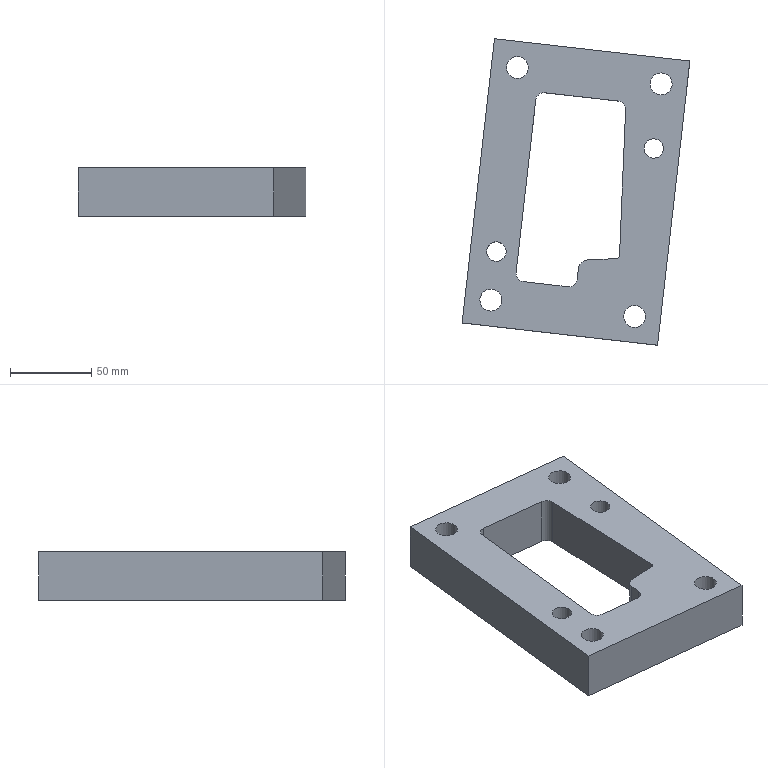Part | NX | features solid 2 | 1 solid | 36 faces | box 140.146 x 188.566 x 30 mm | volume 409846 mm3 | cylinder 18 | plane 17 | spline 1 | commonest cylinder face diameters 10 x4 13.5 x4 20 x4 12.001 x2 14.11 x2 4 x1
STEP:
#1=CARTESIAN_POINT('',(2935.529,-339.708,61.));
#2=VERTEX_POINT('',#1);
#3=CARTESIAN_POINT('',(2928.474,-339.708,61.));
#4=DIRECTION('',(0.,0.,1.));
#5=DIRECTION('',(1.,0.,0.));
#6=AXIS2_PLACEMENT_3D('',#3,#4,#5);
#7=CIRCLE('',#6,7.055);
#8=EDGE_CURVE('',#2,#2,#7,.T.);
#9=ORIENTED_EDGE('',*,*,#8,.T.);
#10=EDGE_LOOP('',(#9));
#11=FACE_BOUND('',#10,.T.);
#12=CARTESIAN_POINT('',(3032.334,-276.258,61.));
#13=VERTEX_POINT('',#12);
#14=CARTESIAN_POINT('',(3025.279,-276.258,61.));
#15=DIRECTION('',(0.,0.,1.));
#16=DIRECTION('',(1.,0.,0.));
#17=AXIS2_PLACEMENT_3D('',#14,#15,#16);
#18=CIRCLE('',#17,7.055);
#19=EDGE_CURVE('',#13,#13,#18,.T.);
#20=ORIENTED_EDGE('',*,*,#19,.T.);
#21=EDGE_LOOP('',(#20));
#22=FACE_BOUND('',#21,.T.);
#23=CARTESIAN_POINT('',(2951.315,-227.572,61.));
#24=VERTEX_POINT('',#23);
#25=CARTESIAN_POINT('',(2941.379,-226.44,61.));
#26=DIRECTION('',(0.,0.,1.));
#27=DIRECTION('',(0.9936,-0.1132,0.));
#28=AXIS2_PLACEMENT_3D('',#25,#26,#27);
#29=CIRCLE('',#28,10.);
#30=EDGE_CURVE('',#24,#24,#29,.T.);
#31=ORIENTED_EDGE('',*,*,#30,.T.);
#32=EDGE_LOOP('',(#31));
#33=FACE_BOUND('',#32,.T.);
#34=CARTESIAN_POINT('',(3039.743,-237.647,61.));
#35=VERTEX_POINT('',#34);
#36=CARTESIAN_POINT('',(3029.807,-236.515,61.));
#37=DIRECTION('',(0.,0.,1.));
#38=DIRECTION('',(0.9936,-0.1132,0.));
#39=AXIS2_PLACEMENT_3D('',#36,#37,#38);
#40=CIRCLE('',#39,10.);
#41=EDGE_CURVE('',#35,#35,#40,.T.);
#42=ORIENTED_EDGE('',*,*,#41,.T.);
#43=EDGE_LOOP('',(#42));
#44=FACE_BOUND('',#43,.T.);
#45=CARTESIAN_POINT('',(3027.592,-397.298,61.));
#46=VERTEX_POINT('',#45);
#47=CARTESIAN_POINT('',(3047.516,-222.43,61.));
#48=VERTEX_POINT('',#47);
#49=CARTESIAN_POINT('',(3037.554,-309.864,61.));
#50=DIRECTION('',(0.1132,0.9936,0.));
#51=VECTOR('',#50,1000.);
#52=LINE('',#49,#51);
#53=EDGE_CURVE('',#46,#48,#52,.T.);
#54=ORIENTED_EDGE('',*,*,#53,.F.);
#55=CARTESIAN_POINT('',(2907.37,-383.601,61.));
#56=VERTEX_POINT('',#55);
#57=CARTESIAN_POINT('',(2967.481,-390.449,61.));
#58=DIRECTION('',(0.9936,-0.1132,0.));
#59=VECTOR('',#58,1000.);
#60=LINE('',#57,#59);
#61=EDGE_CURVE('',#56,#46,#60,.T.);
#62=ORIENTED_EDGE('',*,*,#61,.F.);
#63=CARTESIAN_POINT('',(2927.293,-208.732,61.));
#64=VERTEX_POINT('',#63);
#65=CARTESIAN_POINT('',(2917.331,-296.166,61.));
#66=DIRECTION('',(-0.1132,-0.9936,0.));
#67=VECTOR('',#66,1000.);
#68=LINE('',#65,#67);
#69=EDGE_CURVE('',#64,#56,#68,.T.);
#70=ORIENTED_EDGE('',*,*,#69,.F.);
#71=CARTESIAN_POINT('',(2987.404,-215.581,61.));
#72=DIRECTION('',(-0.9936,0.1132,0.));
#73=VECTOR('',#72,1000.);
#74=LINE('',#71,#73);
#75=EDGE_CURVE('',#48,#64,#74,.T.);
#76=ORIENTED_EDGE('',*,*,#75,.F.);
#77=EDGE_LOOP('',(#54,#62,#70,#76));
#78=FACE_BOUND('',#77,.T.);
#79=CARTESIAN_POINT('',(2935.014,-370.647,61.));
#80=VERTEX_POINT('',#79);
#81=CARTESIAN_POINT('',(2925.078,-369.515,61.));
#82=DIRECTION('',(0.,0.,1.));
#83=DIRECTION('',(0.9936,-0.1132,0.));
#84=AXIS2_PLACEMENT_3D('',#81,#82,#83);
#85=CIRCLE('',#84,10.);
#86=EDGE_CURVE('',#80,#80,#85,.T.);
#87=ORIENTED_EDGE('',*,*,#86,.T.);
#88=EDGE_LOOP('',(#87));
#89=FACE_BOUND('',#88,.T.);
#90=CARTESIAN_POINT('',(3023.442,-380.722,61.));
#91=VERTEX_POINT('',#90);
#92=CARTESIAN_POINT('',(3013.506,-379.59,61.));
#93=DIRECTION('',(0.,0.,1.));
#94=DIRECTION('',(0.9936,-0.1132,0.));
#95=AXIS2_PLACEMENT_3D('',#92,#93,#94);
#96=CIRCLE('',#95,10.);
#97=EDGE_CURVE('',#91,#91,#96,.T.);
#98=ORIENTED_EDGE('',*,*,#97,.T.);
#99=EDGE_LOOP('',(#98));
#100=FACE_BOUND('',#99,.T.);
#101=CARTESIAN_POINT('',(3002.271,-343.982,61.));
#102=VERTEX_POINT('',#101);
#103=CARTESIAN_POINT('',(3004.206,-342.067,61.));
#104=VERTEX_POINT('',#103);
#105=CARTESIAN_POINT('',(3002.208,-341.983,61.));
#106=DIRECTION('',(0.,0.,1.));
#107=DIRECTION('',(-1.,0.,0.));
#108=AXIS2_PLACEMENT_3D('',#105,#106,#107);
#109=CIRCLE('',#108,2.);
#110=EDGE_CURVE('',#102,#104,#109,.T.);
#111=ORIENTED_EDGE('',*,*,#110,.T.);
#112=CARTESIAN_POINT('',(3007.966,-252.287,61.));
#113=VERTEX_POINT('',#112);
#114=CARTESIAN_POINT('',(3005.792,-304.202,61.));
#115=DIRECTION('',(0.04184,0.9991,0.));
#116=VECTOR('',#115,1000.);
#117=LINE('',#114,#116);
#118=EDGE_CURVE('',#104,#113,#117,.T.);
#119=ORIENTED_EDGE('',*,*,#118,.T.);
#120=CARTESIAN_POINT('',(3003.536,-247.11,61.));
#121=VERTEX_POINT('',#120);
#122=CARTESIAN_POINT('',(3002.97,-252.077,61.));
#123=DIRECTION('',(0.,0.,-1.));
#124=DIRECTION('',(-1.,0.,0.));
#125=AXIS2_PLACEMENT_3D('',#122,#123,#124);
#126=CIRCLE('',#125,5.);
#127=EDGE_CURVE('',#121,#113,#126,.T.);
#128=ORIENTED_EDGE('',*,*,#127,.F.);
#129=CARTESIAN_POINT('',(2958.215,-241.946,61.));
#130=VERTEX_POINT('',#129);
#131=CARTESIAN_POINT('',(2984.065,-244.891,61.));
#132=DIRECTION('',(0.9936,-0.1132,0.));
#133=VECTOR('',#132,1000.);
#134=LINE('',#131,#133);
#135=EDGE_CURVE('',#130,#121,#134,.T.);
#136=ORIENTED_EDGE('',*,*,#135,.F.);
#137=CARTESIAN_POINT('',(2952.681,-246.348,61.));
#138=VERTEX_POINT('',#137);
#139=CARTESIAN_POINT('',(2957.649,-246.914,61.));
#140=DIRECTION('',(0.,0.,-1.));
#141=DIRECTION('',(-1.,0.,0.));
#142=AXIS2_PLACEMENT_3D('',#139,#140,#141);
#143=CIRCLE('',#142,5.);
#144=EDGE_CURVE('',#138,#130,#143,.T.);
#145=ORIENTED_EDGE('',*,*,#144,.F.);
#146=CARTESIAN_POINT('',(2940.568,-352.66,61.));
#147=VERTEX_POINT('',#146);
#148=CARTESIAN_POINT('',(2946.624,-299.504,61.));
#149=DIRECTION('',(0.1132,0.9936,0.));
#150=VECTOR('',#149,1000.);
#151=LINE('',#148,#150);
#152=EDGE_CURVE('',#147,#138,#151,.T.);
#153=ORIENTED_EDGE('',*,*,#152,.F.);
#154=CARTESIAN_POINT('',(2944.97,-358.194,61.));
#155=VERTEX_POINT('',#154);
#156=CARTESIAN_POINT('',(2945.536,-353.226,61.));
#157=DIRECTION('',(0.,0.,-1.));
#158=DIRECTION('',(-1.,0.,0.));
#159=AXIS2_PLACEMENT_3D('',#156,#157,#158);
#160=CIRCLE('',#159,5.);
#161=EDGE_CURVE('',#155,#147,#160,.T.);
#162=ORIENTED_EDGE('',*,*,#161,.F.);
#163=CARTESIAN_POINT('',(2972.614,-361.343,61.));
#164=VERTEX_POINT('',#163);
#165=CARTESIAN_POINT('',(2970.82,-361.139,61.));
#166=DIRECTION('',(-0.9936,0.1132,0.));
#167=VECTOR('',#166,1000.);
#168=LINE('',#165,#167);
#169=EDGE_CURVE('',#164,#155,#168,.T.);
#170=ORIENTED_EDGE('',*,*,#169,.F.);
#171=CARTESIAN_POINT('',(2978.148,-356.942,61.));
#172=VERTEX_POINT('',#171);
#173=CARTESIAN_POINT('',(2973.18,-356.376,61.));
#174=DIRECTION('',(0.,0.,-1.));
#175=DIRECTION('',(-1.,0.,0.));
#176=AXIS2_PLACEMENT_3D('',#173,#174,#175);
#177=CIRCLE('',#176,5.);
#178=EDGE_CURVE('',#172,#164,#177,.T.);
#179=ORIENTED_EDGE('',*,*,#178,.F.);
#180=CARTESIAN_POINT('',(2978.919,-350.168,61.));
#181=VERTEX_POINT('',#180);
#182=CARTESIAN_POINT('',(2984.204,-303.785,61.));
#183=DIRECTION('',(0.1132,0.9936,0.));
#184=VECTOR('',#183,1000.);
#185=LINE('',#182,#184);
#186=EDGE_CURVE('',#172,#181,#185,.T.);
#187=ORIENTED_EDGE('',*,*,#186,.T.);
#188=CARTESIAN_POINT('',(2984.567,-344.856,61.));
#189=VERTEX_POINT('',#188);
#190=CARTESIAN_POINT('',(2984.881,-350.848,61.));
#191=DIRECTION('',(0.,0.,-1.));
#192=DIRECTION('',(-1.,0.,0.));
#193=AXIS2_PLACEMENT_3D('',#190,#191,#192);
#194=CIRCLE('',#193,6.);
#195=EDGE_CURVE('',#181,#189,#194,.T.);
#196=ORIENTED_EDGE('',*,*,#195,.T.);
#197=CARTESIAN_POINT('',(2984.567,-344.856,61.));
#198=CARTESIAN_POINT('',(2990.468,-344.547,61.));
#199=CARTESIAN_POINT('',(2996.365,-344.168,61.));
#200=CARTESIAN_POINT('',(3002.271,-343.982,61.));
#201=B_SPLINE_CURVE_WITH_KNOTS('',3,(#197,#198,#199,#200),.UNSPECIFIED.,.F.,.F.,(4,4),(0.,0.01773),.UNSPECIFIED.);
#202=EDGE_CURVE('',#189,#102,#201,.T.);
#203=ORIENTED_EDGE('',*,*,#202,.T.);
#204=EDGE_LOOP('',(#111,#119,#128,#136,#145,#153,#162,#170,#179,#187,#196,#203));
#205=FACE_BOUND('',#204,.T.);
#206=CARTESIAN_POINT('',(2977.443,-303.015,61.));
#207=DIRECTION('',(0.,0.,-1.));
#208=DIRECTION('',(0.9936,-0.1132,0.));
#209=AXIS2_PLACEMENT_3D('',#206,#207,#208);
#210=PLANE('',#209);
#211=ADVANCED_FACE('',(#11,#22,#33,#44,#78,#89,#100,#205),#210,.T.);
#212=CARTESIAN_POINT('',(3027.592,-397.298,91.));
#213=VERTEX_POINT('',#212);
#214=CARTESIAN_POINT('',(2907.37,-383.601,91.));
#215=VERTEX_POINT('',#214);
#216=CARTESIAN_POINT('',(2967.481,-390.449,91.));
#217=DIRECTION('',(-0.9936,0.1132,0.));
#218=VECTOR('',#217,1000.);
#219=LINE('',#216,#218);
#220=EDGE_CURVE('',#213,#215,#219,.T.);
#221=ORIENTED_EDGE('',*,*,#220,.F.);
#222=CARTESIAN_POINT('',(3047.516,-222.43,91.));
#223=VERTEX_POINT('',#222);
#224=CARTESIAN_POINT('',(3037.554,-309.864,91.));
#225=DIRECTION('',(-0.1132,-0.9936,0.));
#226=VECTOR('',#225,1000.);
#227=LINE('',#224,#226);
#228=EDGE_CURVE('',#223,#213,#227,.T.);
#229=ORIENTED_EDGE('',*,*,#228,.F.);
#230=CARTESIAN_POINT('',(2927.293,-208.732,91.));
#231=VERTEX_POINT('',#230);
#232=CARTESIAN_POINT('',(2987.404,-215.581,91.));
#233=DIRECTION('',(0.9936,-0.1132,0.));
#234=VECTOR('',#233,1000.);
#235=LINE('',#232,#234);
#236=EDGE_CURVE('',#231,#223,#235,.T.);
#237=ORIENTED_EDGE('',*,*,#236,.F.);
#238=CARTESIAN_POINT('',(2917.331,-296.166,91.));
#239=DIRECTION('',(0.1132,0.9936,0.));
#240=VECTOR('',#239,1000.);
#241=LINE('',#238,#240);
#242=EDGE_CURVE('',#215,#231,#241,.T.);
#243=ORIENTED_EDGE('',*,*,#242,.F.);
#244=EDGE_LOOP('',(#221,#229,#237,#243));
#245=FACE_BOUND('',#244,.T.);
#246=CARTESIAN_POINT('',(2931.785,-370.279,91.));
#247=VERTEX_POINT('',#246);
#248=CARTESIAN_POINT('',(2925.078,-369.515,91.));
#249=DIRECTION('',(0.,0.,1.));
#250=DIRECTION('',(0.9936,-0.1132,0.));
#251=AXIS2_PLACEMENT_3D('',#248,#249,#250);
#252=CIRCLE('',#251,6.75);
#253=EDGE_CURVE('',#247,#247,#252,.T.);
#254=ORIENTED_EDGE('',*,*,#253,.F.);
#255=EDGE_LOOP('',(#254));
#256=FACE_BOUND('',#255,.T.);
#257=CARTESIAN_POINT('',(3036.514,-237.28,91.));
#258=VERTEX_POINT('',#257);
#259=CARTESIAN_POINT('',(3029.807,-236.515,91.));
#260=DIRECTION('',(0.,0.,1.));
#261=DIRECTION('',(0.9936,-0.1132,0.));
#262=AXIS2_PLACEMENT_3D('',#259,#260,#261);
#263=CIRCLE('',#262,6.75);
#264=EDGE_CURVE('',#258,#258,#263,.T.);
#265=ORIENTED_EDGE('',*,*,#264,.F.);
#266=EDGE_LOOP('',(#265));
#267=FACE_BOUND('',#266,.T.);
#268=CARTESIAN_POINT('',(3020.212,-380.354,91.));
#269=VERTEX_POINT('',#268);
#270=CARTESIAN_POINT('',(3013.506,-379.59,91.));
#271=DIRECTION('',(0.,0.,1.));
#272=DIRECTION('',(0.9936,-0.1132,0.));
#273=AXIS2_PLACEMENT_3D('',#270,#271,#272);
#274=CIRCLE('',#273,6.75);
#275=EDGE_CURVE('',#269,#269,#274,.T.);
#276=ORIENTED_EDGE('',*,*,#275,.F.);
#277=EDGE_LOOP('',(#276));
#278=FACE_BOUND('',#277,.T.);
#279=CARTESIAN_POINT('',(2948.086,-227.204,91.));
#280=VERTEX_POINT('',#279);
#281=CARTESIAN_POINT('',(2941.379,-226.44,91.));
#282=DIRECTION('',(0.,0.,1.));
#283=DIRECTION('',(0.9936,-0.1132,0.));
#284=AXIS2_PLACEMENT_3D('',#281,#282,#283);
#285=CIRCLE('',#284,6.75);
#286=EDGE_CURVE('',#280,#280,#285,.T.);
#287=ORIENTED_EDGE('',*,*,#286,.F.);
#288=EDGE_LOOP('',(#287));
#289=FACE_BOUND('',#288,.T.);
#290=CARTESIAN_POINT('',(2934.436,-340.387,91.));
#291=VERTEX_POINT('',#290);
#292=CARTESIAN_POINT('',(2928.474,-339.708,91.));
#293=DIRECTION('',(0.,0.,1.));
#294=DIRECTION('',(0.9936,-0.1132,0.));
#295=AXIS2_PLACEMENT_3D('',#292,#293,#294);
#296=CIRCLE('',#295,6.);
#297=EDGE_CURVE('',#291,#291,#296,.T.);
#298=ORIENTED_EDGE('',*,*,#297,.F.);
#299=EDGE_LOOP('',(#298));
#300=FACE_BOUND('',#299,.T.);
#301=CARTESIAN_POINT('',(3031.241,-276.938,91.));
#302=VERTEX_POINT('',#301);
#303=CARTESIAN_POINT('',(3025.279,-276.258,91.));
#304=DIRECTION('',(0.,0.,1.));
#305=DIRECTION('',(0.9936,-0.1132,0.));
#306=AXIS2_PLACEMENT_3D('',#303,#304,#305);
#307=CIRCLE('',#306,6.);
#308=EDGE_CURVE('',#302,#302,#307,.T.);
#309=ORIENTED_EDGE('',*,*,#308,.F.);
#310=EDGE_LOOP('',(#309));
#311=FACE_BOUND('',#310,.T.);
#312=CARTESIAN_POINT('',(2958.215,-241.946,91.));
#313=VERTEX_POINT('',#312);
#314=CARTESIAN_POINT('',(2952.681,-246.348,91.));
#315=VERTEX_POINT('',#314);
#316=CARTESIAN_POINT('',(2957.649,-246.914,91.));
#317=DIRECTION('',(0.,0.,1.));
#318=DIRECTION('',(1.,0.,0.));
#319=AXIS2_PLACEMENT_3D('',#316,#317,#318);
#320=CIRCLE('',#319,5.);
#321=EDGE_CURVE('',#313,#315,#320,.T.);
#322=ORIENTED_EDGE('',*,*,#321,.F.);
#323=CARTESIAN_POINT('',(3003.536,-247.11,91.));
#324=VERTEX_POINT('',#323);
#325=CARTESIAN_POINT('',(2988.519,-245.399,91.));
#326=DIRECTION('',(0.9936,-0.1132,0.));
#327=VECTOR('',#326,1000.);
#328=LINE('',#325,#327);
#329=EDGE_CURVE('',#313,#324,#328,.T.);
#330=ORIENTED_EDGE('',*,*,#329,.T.);
#331=CARTESIAN_POINT('',(3007.966,-252.287,91.));
#332=VERTEX_POINT('',#331);
#333=CARTESIAN_POINT('',(3002.97,-252.077,91.));
#334=DIRECTION('',(0.,0.,1.));
#335=DIRECTION('',(1.,0.,0.));
#336=AXIS2_PLACEMENT_3D('',#333,#334,#335);
#337=CIRCLE('',#336,5.);
#338=EDGE_CURVE('',#332,#324,#337,.T.);
#339=ORIENTED_EDGE('',*,*,#338,.F.);
#340=CARTESIAN_POINT('',(3004.206,-342.067,91.));
#341=VERTEX_POINT('',#340);
#342=CARTESIAN_POINT('',(3007.776,-256.811,91.));
#343=DIRECTION('',(0.04184,0.9991,0.));
#344=VECTOR('',#343,1000.);
#345=LINE('',#342,#344);
#346=EDGE_CURVE('',#341,#332,#345,.T.);
#347=ORIENTED_EDGE('',*,*,#346,.F.);
#348=CARTESIAN_POINT('',(3002.271,-343.982,91.));
#349=VERTEX_POINT('',#348);
#350=CARTESIAN_POINT('',(3002.208,-341.983,91.));
#351=DIRECTION('',(0.,0.,-1.));
#352=DIRECTION('',(1.,0.,0.));
#353=AXIS2_PLACEMENT_3D('',#350,#351,#352);
#354=CIRCLE('',#353,2.);
#355=EDGE_CURVE('',#341,#349,#354,.T.);
#356=ORIENTED_EDGE('',*,*,#355,.T.);
#357=CARTESIAN_POINT('',(2984.567,-344.856,91.));
#358=VERTEX_POINT('',#357);
#359=CARTESIAN_POINT('',(3002.271,-343.982,91.));
#360=CARTESIAN_POINT('',(2996.365,-344.168,91.));
#361=CARTESIAN_POINT('',(2990.468,-344.547,91.));
#362=CARTESIAN_POINT('',(2984.567,-344.856,91.));
#363=B_SPLINE_CURVE_WITH_KNOTS('',3,(#359,#360,#361,#362),.UNSPECIFIED.,.F.,.F.,(4,4),(0.,0.01772),.UNSPECIFIED.);
#364=EDGE_CURVE('',#349,#358,#363,.T.);
#365=ORIENTED_EDGE('',*,*,#364,.T.);
#366=CARTESIAN_POINT('',(2978.919,-350.168,91.));
#367=VERTEX_POINT('',#366);
#368=CARTESIAN_POINT('',(2984.881,-350.848,91.));
#369=DIRECTION('',(0.,0.,1.));
#370=DIRECTION('',(1.,0.,0.));
#371=AXIS2_PLACEMENT_3D('',#368,#369,#370);
#372=CIRCLE('',#371,6.);
#373=EDGE_CURVE('',#358,#367,#372,.T.);
#374=ORIENTED_EDGE('',*,*,#373,.T.);
#375=CARTESIAN_POINT('',(2978.148,-356.942,91.));
#376=VERTEX_POINT('',#375);
#377=CARTESIAN_POINT('',(3005.458,-117.242,91.));
#378=DIRECTION('',(-0.1132,-0.9936,0.));
#379=VECTOR('',#378,1000.);
#380=LINE('',#377,#379);
#381=EDGE_CURVE('',#367,#376,#380,.T.);
#382=ORIENTED_EDGE('',*,*,#381,.T.);
#383=CARTESIAN_POINT('',(2972.614,-361.343,91.));
#384=VERTEX_POINT('',#383);
#385=CARTESIAN_POINT('',(2973.18,-356.376,91.));
#386=DIRECTION('',(0.,0.,1.));
#387=DIRECTION('',(1.,0.,0.));
#388=AXIS2_PLACEMENT_3D('',#385,#386,#387);
#389=CIRCLE('',#388,5.);
#390=EDGE_CURVE('',#384,#376,#389,.T.);
#391=ORIENTED_EDGE('',*,*,#390,.F.);
#392=CARTESIAN_POINT('',(2944.97,-358.194,91.));
#393=VERTEX_POINT('',#392);
#394=CARTESIAN_POINT('',(2975.274,-361.646,91.));
#395=DIRECTION('',(-0.9936,0.1132,0.));
#396=VECTOR('',#395,1000.);
#397=LINE('',#394,#396);
#398=EDGE_CURVE('',#384,#393,#397,.T.);
#399=ORIENTED_EDGE('',*,*,#398,.T.);
#400=CARTESIAN_POINT('',(2940.568,-352.66,91.));
#401=VERTEX_POINT('',#400);
#402=CARTESIAN_POINT('',(2945.536,-353.226,91.));
#403=DIRECTION('',(0.,0.,1.));
#404=DIRECTION('',(1.,0.,0.));
#405=AXIS2_PLACEMENT_3D('',#402,#403,#404);
#406=CIRCLE('',#405,5.);
#407=EDGE_CURVE('',#401,#393,#406,.T.);
#408=ORIENTED_EDGE('',*,*,#407,.F.);
#409=CARTESIAN_POINT('',(2946.568,-300.001,91.));
#410=DIRECTION('',(0.1132,0.9936,0.));
#411=VECTOR('',#410,1000.);
#412=LINE('',#409,#411);
#413=EDGE_CURVE('',#401,#315,#412,.T.);
#414=ORIENTED_EDGE('',*,*,#413,.T.);
#415=EDGE_LOOP('',(#322,#330,#339,#347,#356,#365,#374,#382,#391,#399,#408,#414));
#416=FACE_BOUND('',#415,.T.);
#417=CARTESIAN_POINT('',(2977.443,-303.015,91.));
#418=DIRECTION('',(0.,0.,1.));
#419=DIRECTION('',(-0.9936,0.1132,0.));
#420=AXIS2_PLACEMENT_3D('',#417,#418,#419);
#421=PLANE('',#420);
#422=ADVANCED_FACE('',(#245,#256,#267,#278,#289,#300,#311,#416),#421,.T.);
#423=CARTESIAN_POINT('',(3027.592,-397.298,61.));
#424=DIRECTION('',(0.,0.,1.));
#425=VECTOR('',#424,1000.);
#426=LINE('',#423,#425);
#427=EDGE_CURVE('',#46,#213,#426,.T.);
#428=ORIENTED_EDGE('',*,*,#427,.T.);
#429=ORIENTED_EDGE('',*,*,#220,.T.);
#430=CARTESIAN_POINT('',(2907.37,-383.601,61.));
#431=DIRECTION('',(0.,0.,1.));
#432=VECTOR('',#431,1000.);
#433=LINE('',#430,#432);
#434=EDGE_CURVE('',#56,#215,#433,.T.);
#435=ORIENTED_EDGE('',*,*,#434,.F.);
#436=ORIENTED_EDGE('',*,*,#61,.T.);
#437=EDGE_LOOP('',(#428,#429,#435,#436));
#438=FACE_BOUND('',#437,.T.);
#439=CARTESIAN_POINT('',(2967.481,-390.449,61.));
#440=DIRECTION('',(-0.1132,-0.9936,0.));
#441=DIRECTION('',(0.,0.,1.));
#442=AXIS2_PLACEMENT_3D('',#439,#440,#441);
#443=PLANE('',#442);
#444=ADVANCED_FACE('',(#438),#443,.T.);
#445=ORIENTED_EDGE('',*,*,#434,.T.);
#446=ORIENTED_EDGE('',*,*,#242,.T.);
#447=CARTESIAN_POINT('',(2927.293,-208.732,61.));
#448=DIRECTION('',(0.,0.,1.));
#449=VECTOR('',#448,1000.);
#450=LINE('',#447,#449);
#451=EDGE_CURVE('',#64,#231,#450,.T.);
#452=ORIENTED_EDGE('',*,*,#451,.F.);
#453=ORIENTED_EDGE('',*,*,#69,.T.);
#454=EDGE_LOOP('',(#445,#446,#452,#453));
#455=FACE_BOUND('',#454,.T.);
#456=CARTESIAN_POINT('',(2917.331,-296.166,61.));
#457=DIRECTION('',(-0.9936,0.1132,0.));
#458=DIRECTION('',(0.,0.,-1.));
#459=AXIS2_PLACEMENT_3D('',#456,#457,#458);
#460=PLANE('',#459);
#461=ADVANCED_FACE('',(#455),#460,.T.);
#462=ORIENTED_EDGE('',*,*,#451,.T.);
#463=ORIENTED_EDGE('',*,*,#236,.T.);
#464=CARTESIAN_POINT('',(3047.516,-222.43,61.));
#465=DIRECTION('',(0.,0.,1.));
#466=VECTOR('',#465,1000.);
#467=LINE('',#464,#466);
#468=EDGE_CURVE('',#48,#223,#467,.T.);
#469=ORIENTED_EDGE('',*,*,#468,.F.);
#470=ORIENTED_EDGE('',*,*,#75,.T.);
#471=EDGE_LOOP('',(#462,#463,#469,#470));
#472=FACE_BOUND('',#471,.T.);
#473=CARTESIAN_POINT('',(2987.404,-215.581,61.));
#474=DIRECTION('',(0.1132,0.9936,0.));
#475=DIRECTION('',(0.,0.,-1.));
#476=AXIS2_PLACEMENT_3D('',#473,#474,#475);
#477=PLANE('',#476);
#478=ADVANCED_FACE('',(#472),#477,.T.);
#479=ORIENTED_EDGE('',*,*,#53,.T.);
#480=ORIENTED_EDGE('',*,*,#468,.T.);
#481=ORIENTED_EDGE('',*,*,#228,.T.);
#482=ORIENTED_EDGE('',*,*,#427,.F.);
#483=EDGE_LOOP('',(#479,#480,#481,#482));
#484=FACE_BOUND('',#483,.T.);
#485=CARTESIAN_POINT('',(3037.554,-309.864,61.));
#486=DIRECTION('',(0.9936,-0.1132,0.));
#487=DIRECTION('',(0.,0.,1.));
#488=AXIS2_PLACEMENT_3D('',#485,#486,#487);
#489=PLANE('',#488);
#490=ADVANCED_FACE('',(#484),#489,.T.);
#491=ORIENTED_EDGE('',*,*,#253,.T.);
#492=EDGE_LOOP('',(#491));
#493=FACE_BOUND('',#492,.T.);
#494=CARTESIAN_POINT('',(2931.785,-370.279,76.));
#495=VERTEX_POINT('',#494);
#496=CARTESIAN_POINT('',(2925.078,-369.515,76.));
#497=DIRECTION('',(0.,0.,1.));
#498=DIRECTION('',(0.9936,-0.1132,0.));
#499=AXIS2_PLACEMENT_3D('',#496,#497,#498);
#500=CIRCLE('',#499,6.75);
#501=EDGE_CURVE('',#495,#495,#500,.T.);
#502=ORIENTED_EDGE('',*,*,#501,.F.);
#503=EDGE_LOOP('',(#502));
#504=FACE_BOUND('',#503,.T.);
#505=CARTESIAN_POINT('',(2925.078,-369.515,58.));
#506=DIRECTION('',(0.,0.,1.));
#507=DIRECTION('',(-0.9936,0.1132,0.));
#508=AXIS2_PLACEMENT_3D('',#505,#506,#507);
#509=CYLINDRICAL_SURFACE('',#508,6.75);
#510=ADVANCED_FACE('',(#493,#504),#509,.F.);
#511=ORIENTED_EDGE('',*,*,#501,.T.);
#512=EDGE_LOOP('',(#511));
#513=FACE_BOUND('',#512,.T.);
#514=CARTESIAN_POINT('',(2935.014,-370.647,76.));
#515=VERTEX_POINT('',#514);
#516=CARTESIAN_POINT('',(2925.078,-369.515,76.));
#517=DIRECTION('',(0.,0.,1.));
#518=DIRECTION('',(0.9936,-0.1132,0.));
#519=AXIS2_PLACEMENT_3D('',#516,#517,#518);
#520=CIRCLE('',#519,10.);
#521=EDGE_CURVE('',#515,#515,#520,.T.);
#522=ORIENTED_EDGE('',*,*,#521,.F.);
#523=EDGE_LOOP('',(#522));
#524=FACE_BOUND('',#523,.T.);
#525=CARTESIAN_POINT('',(2925.078,-369.515,76.));
#526=DIRECTION('',(0.,0.,1.));
#527=DIRECTION('',(-0.9936,0.1132,0.));
#528=AXIS2_PLACEMENT_3D('',#525,#526,#527);
#529=PLANE('',#528);
#530=ADVANCED_FACE('',(#513,#524),#529,.F.);
#531=ORIENTED_EDGE('',*,*,#521,.T.);
#532=EDGE_LOOP('',(#531));
#533=FACE_BOUND('',#532,.T.);
#534=ORIENTED_EDGE('',*,*,#86,.F.);
#535=EDGE_LOOP('',(#534));
#536=FACE_BOUND('',#535,.T.);
#537=CARTESIAN_POINT('',(2925.078,-369.515,61.));
#538=DIRECTION('',(0.,0.,1.));
#539=DIRECTION('',(-0.9936,0.1132,0.));
#540=AXIS2_PLACEMENT_3D('',#537,#538,#539);
#541=CYLINDRICAL_SURFACE('',#540,10.);
#542=ADVANCED_FACE('',(#533,#536),#541,.F.);
#543=ORIENTED_EDGE('',*,*,#264,.T.);
#544=EDGE_LOOP('',(#543));
#545=FACE_BOUND('',#544,.T.);
#546=CARTESIAN_POINT('',(3036.514,-237.28,76.));
#547=VERTEX_POINT('',#546);
#548=CARTESIAN_POINT('',(3029.807,-236.515,76.));
#549=DIRECTION('',(0.,0.,1.));
#550=DIRECTION('',(0.9936,-0.1132,0.));
#551=AXIS2_PLACEMENT_3D('',#548,#549,#550);
#552=CIRCLE('',#551,6.75);
#553=EDGE_CURVE('',#547,#547,#552,.T.);
#554=ORIENTED_EDGE('',*,*,#553,.F.);
#555=EDGE_LOOP('',(#554));
#556=FACE_BOUND('',#555,.T.);
#557=CARTESIAN_POINT('',(3029.807,-236.515,58.));
#558=DIRECTION('',(0.,0.,1.));
#559=DIRECTION('',(-0.9936,0.1132,0.));
#560=AXIS2_PLACEMENT_3D('',#557,#558,#559);
#561=CYLINDRICAL_SURFACE('',#560,6.75);
#562=ADVANCED_FACE('',(#545,#556),#561,.F.);
#563=ORIENTED_EDGE('',*,*,#553,.T.);
#564=EDGE_LOOP('',(#563));
#565=FACE_BOUND('',#564,.T.);
#566=CARTESIAN_POINT('',(3039.743,-237.647,76.));
#567=VERTEX_POINT('',#566);
#568=CARTESIAN_POINT('',(3029.807,-236.515,76.));
#569=DIRECTION('',(0.,0.,1.));
#570=DIRECTION('',(0.9936,-0.1132,0.));
#571=AXIS2_PLACEMENT_3D('',#568,#569,#570);
#572=CIRCLE('',#571,10.);
#573=EDGE_CURVE('',#567,#567,#572,.T.);
#574=ORIENTED_EDGE('',*,*,#573,.F.);
#575=EDGE_LOOP('',(#574));
#576=FACE_BOUND('',#575,.T.);
#577=CARTESIAN_POINT('',(3029.807,-236.515,76.));
#578=DIRECTION('',(0.,0.,1.));
#579=DIRECTION('',(-0.9936,0.1132,0.));
#580=AXIS2_PLACEMENT_3D('',#577,#578,#579);
#581=PLANE('',#580);
#582=ADVANCED_FACE('',(#565,#576),#581,.F.);
#583=ORIENTED_EDGE('',*,*,#573,.T.);
#584=EDGE_LOOP('',(#583));
#585=FACE_BOUND('',#584,.T.);
#586=ORIENTED_EDGE('',*,*,#41,.F.);
#587=EDGE_LOOP('',(#586));
#588=FACE_BOUND('',#587,.T.);
#589=CARTESIAN_POINT('',(3029.807,-236.515,61.));
#590=DIRECTION('',(0.,0.,1.));
#591=DIRECTION('',(-0.9936,0.1132,0.));
#592=AXIS2_PLACEMENT_3D('',#589,#590,#591);
#593=CYLINDRICAL_SURFACE('',#592,10.);
#594=ADVANCED_FACE('',(#585,#588),#593,.F.);
#595=ORIENTED_EDGE('',*,*,#275,.T.);
#596=EDGE_LOOP('',(#595));
#597=FACE_BOUND('',#596,.T.);
#598=CARTESIAN_POINT('',(3020.212,-380.354,76.));
#599=VERTEX_POINT('',#598);
#600=CARTESIAN_POINT('',(3013.506,-379.59,76.));
#601=DIRECTION('',(0.,0.,1.));
#602=DIRECTION('',(0.9936,-0.1132,0.));
#603=AXIS2_PLACEMENT_3D('',#600,#601,#602);
#604=CIRCLE('',#603,6.75);
#605=EDGE_CURVE('',#599,#599,#604,.T.);
#606=ORIENTED_EDGE('',*,*,#605,.F.);
#607=EDGE_LOOP('',(#606));
#608=FACE_BOUND('',#607,.T.);
#609=CARTESIAN_POINT('',(3013.506,-379.59,58.));
#610=DIRECTION('',(0.,0.,1.));
#611=DIRECTION('',(-0.9936,0.1132,0.));
#612=AXIS2_PLACEMENT_3D('',#609,#610,#611);
#613=CYLINDRICAL_SURFACE('',#612,6.75);
#614=ADVANCED_FACE('',(#597,#608),#613,.F.);
#615=ORIENTED_EDGE('',*,*,#605,.T.);
#616=EDGE_LOOP('',(#615));
#617=FACE_BOUND('',#616,.T.);
#618=CARTESIAN_POINT('',(3023.442,-380.722,76.));
#619=VERTEX_POINT('',#618);
#620=CARTESIAN_POINT('',(3013.506,-379.59,76.));
#621=DIRECTION('',(0.,0.,1.));
#622=DIRECTION('',(0.9936,-0.1132,0.));
#623=AXIS2_PLACEMENT_3D('',#620,#621,#622);
#624=CIRCLE('',#623,10.);
#625=EDGE_CURVE('',#619,#619,#624,.T.);
#626=ORIENTED_EDGE('',*,*,#625,.F.);
#627=EDGE_LOOP('',(#626));
#628=FACE_BOUND('',#627,.T.);
#629=CARTESIAN_POINT('',(3013.506,-379.59,76.));
#630=DIRECTION('',(0.,0.,1.));
#631=DIRECTION('',(-0.9936,0.1132,0.));
#632=AXIS2_PLACEMENT_3D('',#629,#630,#631);
#633=PLANE('',#632);
#634=ADVANCED_FACE('',(#617,#628),#633,.F.);
#635=ORIENTED_EDGE('',*,*,#625,.T.);
#636=EDGE_LOOP('',(#635));
#637=FACE_BOUND('',#636,.T.);
#638=ORIENTED_EDGE('',*,*,#97,.F.);
#639=EDGE_LOOP('',(#638));
#640=FACE_BOUND('',#639,.T.);
#641=CARTESIAN_POINT('',(3013.506,-379.59,61.));
#642=DIRECTION('',(0.,0.,1.));
#643=DIRECTION('',(-0.9936,0.1132,0.));
#644=AXIS2_PLACEMENT_3D('',#641,#642,#643);
#645=CYLINDRICAL_SURFACE('',#644,10.);
#646=ADVANCED_FACE('',(#637,#640),#645,.F.);
#647=ORIENTED_EDGE('',*,*,#286,.T.);
#648=EDGE_LOOP('',(#647));
#649=FACE_BOUND('',#648,.T.);
#650=CARTESIAN_POINT('',(2948.086,-227.204,76.));
#651=VERTEX_POINT('',#650);
#652=CARTESIAN_POINT('',(2941.379,-226.44,76.));
#653=DIRECTION('',(0.,0.,1.));
#654=DIRECTION('',(0.9936,-0.1132,0.));
#655=AXIS2_PLACEMENT_3D('',#652,#653,#654);
#656=CIRCLE('',#655,6.75);
#657=EDGE_CURVE('',#651,#651,#656,.T.);
#658=ORIENTED_EDGE('',*,*,#657,.F.);
#659=EDGE_LOOP('',(#658));
#660=FACE_BOUND('',#659,.T.);
#661=CARTESIAN_POINT('',(2941.379,-226.44,58.));
#662=DIRECTION('',(0.,0.,1.));
#663=DIRECTION('',(-0.9936,0.1132,0.));
#664=AXIS2_PLACEMENT_3D('',#661,#662,#663);
#665=CYLINDRICAL_SURFACE('',#664,6.75);
#666=ADVANCED_FACE('',(#649,#660),#665,.F.);
#667=ORIENTED_EDGE('',*,*,#657,.T.);
#668=EDGE_LOOP('',(#667));
#669=FACE_BOUND('',#668,.T.);
#670=CARTESIAN_POINT('',(2951.315,-227.572,76.));
#671=VERTEX_POINT('',#670);
#672=CARTESIAN_POINT('',(2941.379,-226.44,76.));
#673=DIRECTION('',(0.,0.,1.));
#674=DIRECTION('',(0.9936,-0.1132,0.));
#675=AXIS2_PLACEMENT_3D('',#672,#673,#674);
#676=CIRCLE('',#675,10.);
#677=EDGE_CURVE('',#671,#671,#676,.T.);
#678=ORIENTED_EDGE('',*,*,#677,.F.);
#679=EDGE_LOOP('',(#678));
#680=FACE_BOUND('',#679,.T.);
#681=CARTESIAN_POINT('',(2941.379,-226.44,76.));
#682=DIRECTION('',(0.,0.,1.));
#683=DIRECTION('',(-0.9936,0.1132,0.));
#684=AXIS2_PLACEMENT_3D('',#681,#682,#683);
#685=PLANE('',#684);
#686=ADVANCED_FACE('',(#669,#680),#685,.F.);
#687=ORIENTED_EDGE('',*,*,#677,.T.);
#688=EDGE_LOOP('',(#687));
#689=FACE_BOUND('',#688,.T.);
#690=ORIENTED_EDGE('',*,*,#30,.F.);
#691=EDGE_LOOP('',(#690));
#692=FACE_BOUND('',#691,.T.);
#693=CARTESIAN_POINT('',(2941.379,-226.44,61.));
#694=DIRECTION('',(0.,0.,1.));
#695=DIRECTION('',(-0.9936,0.1132,0.));
#696=AXIS2_PLACEMENT_3D('',#693,#694,#695);
#697=CYLINDRICAL_SURFACE('',#696,10.);
#698=ADVANCED_FACE('',(#689,#692),#697,.F.);
#699=CARTESIAN_POINT('',(2934.475,-339.708,71.));
#700=VERTEX_POINT('',#699);
#701=CARTESIAN_POINT('',(2928.474,-339.708,71.));
#702=DIRECTION('',(0.,0.,-1.));
#703=DIRECTION('',(1.,0.,0.));
#704=AXIS2_PLACEMENT_3D('',#701,#702,#703);
#705=CIRCLE('',#704,6.);
#706=EDGE_CURVE('',#700,#700,#705,.T.);
#707=ORIENTED_EDGE('',*,*,#706,.T.);
#708=EDGE_LOOP('',(#707));
#709=FACE_BOUND('',#708,.T.);
#710=ORIENTED_EDGE('',*,*,#297,.T.);
#711=EDGE_LOOP('',(#710));
#712=FACE_BOUND('',#711,.T.);
#713=CARTESIAN_POINT('',(2928.474,-339.708,58.));
#714=DIRECTION('',(0.,0.,1.));
#715=DIRECTION('',(-0.9936,0.1132,0.));
#716=AXIS2_PLACEMENT_3D('',#713,#714,#715);
#717=CYLINDRICAL_SURFACE('',#716,6.);
#718=ADVANCED_FACE('',(#709,#712),#717,.F.);
#719=CARTESIAN_POINT('',(3031.279,-276.258,71.));
#720=VERTEX_POINT('',#719);
#721=CARTESIAN_POINT('',(3025.279,-276.258,71.));
#722=DIRECTION('',(0.,0.,-1.));
#723=DIRECTION('',(1.,0.,0.));
#724=AXIS2_PLACEMENT_3D('',#721,#722,#723);
#725=CIRCLE('',#724,6.);
#726=EDGE_CURVE('',#720,#720,#725,.T.);
#727=ORIENTED_EDGE('',*,*,#726,.T.);
#728=EDGE_LOOP('',(#727));
#729=FACE_BOUND('',#728,.T.);
#730=ORIENTED_EDGE('',*,*,#308,.T.);
#731=EDGE_LOOP('',(#730));
#732=FACE_BOUND('',#731,.T.);
#733=CARTESIAN_POINT('',(3025.279,-276.258,58.));
#734=DIRECTION('',(0.,0.,1.));
#735=DIRECTION('',(-0.9936,0.1132,0.));
#736=AXIS2_PLACEMENT_3D('',#733,#734,#735);
#737=CYLINDRICAL_SURFACE('',#736,6.);
#738=ADVANCED_FACE('',(#729,#732),#737,.F.);
#739=ORIENTED_EDGE('',*,*,#144,.T.);
#740=CARTESIAN_POINT('',(2958.215,-241.946,0.));
#741=DIRECTION('',(0.,0.,-1.));
#742=VECTOR('',#741,1000.);
#743=LINE('',#740,#742);
#744=EDGE_CURVE('',#313,#130,#743,.T.);
#745=ORIENTED_EDGE('',*,*,#744,.F.);
#746=ORIENTED_EDGE('',*,*,#321,.T.);
#747=CARTESIAN_POINT('',(2952.681,-246.348,0.));
#748=DIRECTION('',(0.,0.,1.));
#749=VECTOR('',#748,1000.);
#750=LINE('',#747,#749);
#751=EDGE_CURVE('',#138,#315,#750,.T.);
#752=ORIENTED_EDGE('',*,*,#751,.F.);
#753=EDGE_LOOP('',(#739,#745,#746,#752));
#754=FACE_BOUND('',#753,.T.);
#755=CARTESIAN_POINT('',(2957.649,-246.914,0.));
#756=DIRECTION('',(0.,0.,1.));
#757=DIRECTION('',(-1.,0.,0.));
#758=AXIS2_PLACEMENT_3D('',#755,#756,#757);
#759=CYLINDRICAL_SURFACE('',#758,5.);
#760=ADVANCED_FACE('',(#754),#759,.F.);
#761=ORIENTED_EDGE('',*,*,#161,.T.);
#762=CARTESIAN_POINT('',(2940.568,-352.66,0.));
#763=DIRECTION('',(0.,0.,-1.));
#764=VECTOR('',#763,1000.);
#765=LINE('',#762,#764);
#766=EDGE_CURVE('',#401,#147,#765,.T.);
#767=ORIENTED_EDGE('',*,*,#766,.F.);
#768=ORIENTED_EDGE('',*,*,#407,.T.);
#769=CARTESIAN_POINT('',(2944.97,-358.194,0.));
#770=DIRECTION('',(0.,0.,1.));
#771=VECTOR('',#770,1000.);
#772=LINE('',#769,#771);
#773=EDGE_CURVE('',#155,#393,#772,.T.);
#774=ORIENTED_EDGE('',*,*,#773,.F.);
#775=EDGE_LOOP('',(#761,#767,#768,#774));
#776=FACE_BOUND('',#775,.T.);
#777=CARTESIAN_POINT('',(2945.536,-353.226,0.));
#778=DIRECTION('',(0.,0.,1.));
#779=DIRECTION('',(-1.,0.,0.));
#780=AXIS2_PLACEMENT_3D('',#777,#778,#779);
#781=CYLINDRICAL_SURFACE('',#780,5.);
#782=ADVANCED_FACE('',(#776),#781,.F.);
#783=ORIENTED_EDGE('',*,*,#152,.T.);
#784=ORIENTED_EDGE('',*,*,#751,.T.);
#785=ORIENTED_EDGE('',*,*,#413,.F.);
#786=ORIENTED_EDGE('',*,*,#766,.T.);
#787=EDGE_LOOP('',(#783,#784,#785,#786));
#788=FACE_BOUND('',#787,.T.);
#789=CARTESIAN_POINT('',(2946.568,-300.001,0.));
#790=DIRECTION('',(-0.9936,0.1132,0.));
#791=DIRECTION('',(0.,0.,-1.));
#792=AXIS2_PLACEMENT_3D('',#789,#790,#791);
#793=PLANE('',#792);
#794=ADVANCED_FACE('',(#788),#793,.F.);
#795=ORIENTED_EDGE('',*,*,#135,.T.);
#796=CARTESIAN_POINT('',(3003.536,-247.11,0.));
#797=DIRECTION('',(0.,0.,1.));
#798=VECTOR('',#797,1000.);
#799=LINE('',#796,#798);
#800=EDGE_CURVE('',#121,#324,#799,.T.);
#801=ORIENTED_EDGE('',*,*,#800,.T.);
#802=ORIENTED_EDGE('',*,*,#329,.F.);
#803=ORIENTED_EDGE('',*,*,#744,.T.);
#804=EDGE_LOOP('',(#795,#801,#802,#803));
#805=FACE_BOUND('',#804,.T.);
#806=CARTESIAN_POINT('',(2988.519,-245.399,0.));
#807=DIRECTION('',(0.1132,0.9936,0.));
#808=DIRECTION('',(0.,0.,-1.));
#809=AXIS2_PLACEMENT_3D('',#806,#807,#808);
#810=PLANE('',#809);
#811=ADVANCED_FACE('',(#805),#810,.F.);
#812=ORIENTED_EDGE('',*,*,#169,.T.);
#813=ORIENTED_EDGE('',*,*,#773,.T.);
#814=ORIENTED_EDGE('',*,*,#398,.F.);
#815=CARTESIAN_POINT('',(2972.614,-361.343,100.));
#816=DIRECTION('',(0.,0.,-1.));
#817=VECTOR('',#816,1000.);
#818=LINE('',#815,#817);
#819=EDGE_CURVE('',#384,#164,#818,.T.);
#820=ORIENTED_EDGE('',*,*,#819,.T.);
#821=EDGE_LOOP('',(#812,#813,#814,#820));
#822=FACE_BOUND('',#821,.T.);
#823=CARTESIAN_POINT('',(2975.274,-361.646,0.));
#824=DIRECTION('',(-0.1132,-0.9936,0.));
#825=DIRECTION('',(0.,0.,1.));
#826=AXIS2_PLACEMENT_3D('',#823,#824,#825);
#827=PLANE('',#826);
#828=ADVANCED_FACE('',(#822),#827,.F.);
#829=ORIENTED_EDGE('',*,*,#178,.T.);
#830=ORIENTED_EDGE('',*,*,#819,.F.);
#831=ORIENTED_EDGE('',*,*,#390,.T.);
#832=CARTESIAN_POINT('',(2978.148,-356.942,0.));
#833=DIRECTION('',(0.,0.,1.));
#834=VECTOR('',#833,1000.);
#835=LINE('',#832,#834);
#836=EDGE_CURVE('',#172,#376,#835,.T.);
#837=ORIENTED_EDGE('',*,*,#836,.F.);
#838=EDGE_LOOP('',(#829,#830,#831,#837));
#839=FACE_BOUND('',#838,.T.);
#840=CARTESIAN_POINT('',(2973.18,-356.376,-404.197));
#841=DIRECTION('',(0.,0.,1.));
#842=DIRECTION('',(-1.,0.,0.));
#843=AXIS2_PLACEMENT_3D('',#840,#841,#842);
#844=CYLINDRICAL_SURFACE('',#843,5.);
#845=ADVANCED_FACE('',(#839),#844,.F.);
#846=ORIENTED_EDGE('',*,*,#836,.T.);
#847=ORIENTED_EDGE('',*,*,#381,.F.);
#848=CARTESIAN_POINT('',(2978.919,-350.168,-404.197));
#849=DIRECTION('',(0.,0.,1.));
#850=VECTOR('',#849,1000.);
#851=LINE('',#848,#850);
#852=EDGE_CURVE('',#181,#367,#851,.T.);
#853=ORIENTED_EDGE('',*,*,#852,.F.);
#854=ORIENTED_EDGE('',*,*,#186,.F.);
#855=EDGE_LOOP('',(#846,#847,#853,#854));
#856=FACE_BOUND('',#855,.T.);
#857=CARTESIAN_POINT('',(2978.919,-350.168,-404.197));
#858=DIRECTION('',(-0.9936,0.1132,0.));
#859=DIRECTION('',(0.1132,0.9936,0.));
#860=AXIS2_PLACEMENT_3D('',#857,#858,#859);
#861=PLANE('',#860);
#862=ADVANCED_FACE('',(#856),#861,.T.);
#863=ORIENTED_EDGE('',*,*,#852,.T.);
#864=ORIENTED_EDGE('',*,*,#373,.F.);
#865=CARTESIAN_POINT('',(2984.567,-344.856,-402.849));
#866=DIRECTION('',(0.,0.,1.));
#867=VECTOR('',#866,1000.);
#868=LINE('',#865,#867);
#869=EDGE_CURVE('',#189,#358,#868,.T.);
#870=ORIENTED_EDGE('',*,*,#869,.F.);
#871=ORIENTED_EDGE('',*,*,#195,.F.);
#872=EDGE_LOOP('',(#863,#864,#870,#871));
#873=FACE_BOUND('',#872,.T.);
#874=CARTESIAN_POINT('',(2984.881,-350.848,-404.197));
#875=DIRECTION('',(0.,0.,1.));
#876=DIRECTION('',(-1.,0.,0.));
#877=AXIS2_PLACEMENT_3D('',#874,#875,#876);
#878=CYLINDRICAL_SURFACE('',#877,6.);
#879=ADVANCED_FACE('',(#873),#878,.T.);
#880=ORIENTED_EDGE('',*,*,#869,.T.);
#881=ORIENTED_EDGE('',*,*,#364,.F.);
#882=CARTESIAN_POINT('',(3002.271,-343.982,-402.195));
#883=DIRECTION('',(0.,0.,1.));
#884=VECTOR('',#883,1000.);
#885=LINE('',#882,#884);
#886=EDGE_CURVE('',#102,#349,#885,.T.);
#887=ORIENTED_EDGE('',*,*,#886,.F.);
#888=ORIENTED_EDGE('',*,*,#202,.F.);
#889=EDGE_LOOP('',(#880,#881,#887,#888));
#890=FACE_BOUND('',#889,.T.);
#891=CARTESIAN_POINT('',(3002.271,-343.982,60.816));
#892=CARTESIAN_POINT('',(3002.271,-343.982,91.838));
#893=CARTESIAN_POINT('',(2996.364,-344.168,60.622));
#894=CARTESIAN_POINT('',(2996.364,-344.168,91.644));
#895=CARTESIAN_POINT('',(2990.468,-344.547,60.384));
#896=CARTESIAN_POINT('',(2990.468,-344.547,91.406));
#897=CARTESIAN_POINT('',(2984.567,-344.856,60.162));
#898=CARTESIAN_POINT('',(2984.567,-344.856,91.184));
#899=B_SPLINE_SURFACE_WITH_KNOTS('',3,1,((#891,#892),(#893,#894),(#895,#896),(#897,#898)),.SURF_OF_LINEAR_EXTRUSION.,.F.,.F.,.F.,(4,4),(2,2),(0.,1.),(0.,1.),.PIECEWISE_BEZIER_KNOTS.);
#900=ADVANCED_FACE('',(#890),#899,.T.);
#901=ORIENTED_EDGE('',*,*,#886,.T.);
#902=ORIENTED_EDGE('',*,*,#355,.F.);
#903=CARTESIAN_POINT('',(3004.206,-342.067,-401.711));
#904=DIRECTION('',(0.,0.,1.));
#905=VECTOR('',#904,1000.);
#906=LINE('',#903,#905);
#907=EDGE_CURVE('',#104,#341,#906,.T.);
#908=ORIENTED_EDGE('',*,*,#907,.F.);
#909=ORIENTED_EDGE('',*,*,#110,.F.);
#910=EDGE_LOOP('',(#901,#902,#908,#909));
#911=FACE_BOUND('',#910,.T.);
#912=CARTESIAN_POINT('',(3002.208,-341.983,-401.744));
#913=DIRECTION('',(0.,0.,1.));
#914=DIRECTION('',(-1.,0.,0.));
#915=AXIS2_PLACEMENT_3D('',#912,#913,#914);
#916=CYLINDRICAL_SURFACE('',#915,2.);
#917=ADVANCED_FACE('',(#911),#916,.F.);
#918=ORIENTED_EDGE('',*,*,#907,.T.);
#919=ORIENTED_EDGE('',*,*,#346,.T.);
#920=CARTESIAN_POINT('',(3007.966,-252.287,100.));
#921=DIRECTION('',(0.,0.,-1.));
#922=VECTOR('',#921,1000.);
#923=LINE('',#920,#922);
#924=EDGE_CURVE('',#332,#113,#923,.T.);
#925=ORIENTED_EDGE('',*,*,#924,.T.);
#926=ORIENTED_EDGE('',*,*,#118,.F.);
#927=EDGE_LOOP('',(#918,#919,#925,#926));
#928=FACE_BOUND('',#927,.T.);
#929=CARTESIAN_POINT('',(3007.776,-256.811,-382.321));
#930=DIRECTION('',(-0.9991,0.04184,0.));
#931=DIRECTION('',(0.04184,0.9991,0.));
#932=AXIS2_PLACEMENT_3D('',#929,#930,#931);
#933=PLANE('',#932);
#934=ADVANCED_FACE('',(#928),#933,.T.);
#935=ORIENTED_EDGE('',*,*,#127,.T.);
#936=ORIENTED_EDGE('',*,*,#924,.F.);
#937=ORIENTED_EDGE('',*,*,#338,.T.);
#938=ORIENTED_EDGE('',*,*,#800,.F.);
#939=EDGE_LOOP('',(#935,#936,#937,#938));
#940=FACE_BOUND('',#939,.T.);
#941=CARTESIAN_POINT('',(3002.97,-252.077,0.));
#942=DIRECTION('',(0.,0.,1.));
#943=DIRECTION('',(-1.,0.,0.));
#944=AXIS2_PLACEMENT_3D('',#941,#942,#943);
#945=CYLINDRICAL_SURFACE('',#944,5.);
#946=ADVANCED_FACE('',(#940),#945,.F.);
#947=CARTESIAN_POINT('',(3032.334,-276.258,71.));
#948=VERTEX_POINT('',#947);
#949=CARTESIAN_POINT('',(3025.279,-276.258,71.));
#950=DIRECTION('',(0.,0.,-1.));
#951=DIRECTION('',(1.,0.,0.));
#952=AXIS2_PLACEMENT_3D('',#949,#950,#951);
#953=CIRCLE('',#952,7.055);
#954=EDGE_CURVE('',#948,#948,#953,.T.);
#955=ORIENTED_EDGE('',*,*,#954,.T.);
#956=EDGE_LOOP('',(#955));
#957=FACE_BOUND('',#956,.T.);
#958=ORIENTED_EDGE('',*,*,#726,.F.);
#959=EDGE_LOOP('',(#958));
#960=FACE_BOUND('',#959,.T.);
#961=CARTESIAN_POINT('',(3025.279,-276.258,71.));
#962=DIRECTION('',(0.,0.,1.));
#963=DIRECTION('',(-1.,0.,0.));
#964=AXIS2_PLACEMENT_3D('',#961,#962,#963);
#965=PLANE('',#964);
#966=ADVANCED_FACE('',(#957,#960),#965,.F.);
#967=ORIENTED_EDGE('',*,*,#954,.F.);
#968=EDGE_LOOP('',(#967));
#969=FACE_BOUND('',#968,.T.);
#970=ORIENTED_EDGE('',*,*,#19,.F.);
#971=EDGE_LOOP('',(#970));
#972=FACE_BOUND('',#971,.T.);
#973=CARTESIAN_POINT('',(3025.279,-276.258,61.));
#974=DIRECTION('',(0.,0.,1.));
#975=DIRECTION('',(-1.,0.,0.));
#976=AXIS2_PLACEMENT_3D('',#973,#974,#975);
#977=CYLINDRICAL_SURFACE('',#976,7.055);
#978=ADVANCED_FACE('',(#969,#972),#977,.F.);
#979=CARTESIAN_POINT('',(2935.529,-339.708,71.));
#980=VERTEX_POINT('',#979);
#981=CARTESIAN_POINT('',(2928.474,-339.708,71.));
#982=DIRECTION('',(0.,0.,-1.));
#983=DIRECTION('',(1.,0.,0.));
#984=AXIS2_PLACEMENT_3D('',#981,#982,#983);
#985=CIRCLE('',#984,7.055);
#986=EDGE_CURVE('',#980,#980,#985,.T.);
#987=ORIENTED_EDGE('',*,*,#986,.T.);
#988=EDGE_LOOP('',(#987));
#989=FACE_BOUND('',#988,.T.);
#990=ORIENTED_EDGE('',*,*,#706,.F.);
#991=EDGE_LOOP('',(#990));
#992=FACE_BOUND('',#991,.T.);
#993=CARTESIAN_POINT('',(2928.474,-339.708,71.));
#994=DIRECTION('',(0.,0.,1.));
#995=DIRECTION('',(-1.,0.,0.));
#996=AXIS2_PLACEMENT_3D('',#993,#994,#995);
#997=PLANE('',#996);
#998=ADVANCED_FACE('',(#989,#992),#997,.F.);
#999=ORIENTED_EDGE('',*,*,#986,.F.);
#1000=EDGE_LOOP('',(#999));
#1001=FACE_BOUND('',#1000,.T.);
#1002=ORIENTED_EDGE('',*,*,#8,.F.);
#1003=EDGE_LOOP('',(#1002));
#1004=FACE_BOUND('',#1003,.T.);
#1005=CARTESIAN_POINT('',(2928.474,-339.708,61.));
#1006=DIRECTION('',(0.,0.,1.));
#1007=DIRECTION('',(-1.,0.,0.));
#1008=AXIS2_PLACEMENT_3D('',#1005,#1006,#1007);
#1009=CYLINDRICAL_SURFACE('',#1008,7.055);
#1010=ADVANCED_FACE('',(#1001,#1004),#1009,.F.);
#1011=CLOSED_SHELL('',(#211,#422,#444,#461,#478,#490,#510,#530,#542,#562,#582,#594,#614,#634,#646,#666,#686,#698,#718,#738,#760,#782,#794,#811,#828,#845,#862,#879,#900,#917,#934,#946,#966,#978,#998,#1010));
#1012=MANIFOLD_SOLID_BREP('',#1011);
#1013=(LENGTH_UNIT()NAMED_UNIT(*)SI_UNIT(.MILLI.,.METRE.));
#1014=UNCERTAINTY_MEASURE_WITH_UNIT(LENGTH_MEASURE(0.0508),#1013,'','');
#1015=(NAMED_UNIT(*)PLANE_ANGLE_UNIT()SI_UNIT($,.RADIAN.));
#1016=(NAMED_UNIT(*)SI_UNIT($,.STERADIAN.)SOLID_ANGLE_UNIT());
#1017=(GEOMETRIC_REPRESENTATION_CONTEXT(3)GLOBAL_UNCERTAINTY_ASSIGNED_CONTEXT((#1014))GLOBAL_UNIT_ASSIGNED_CONTEXT((#1013,#1015,#1016))REPRESENTATION_CONTEXT('',''));
#1018=ADVANCED_BREP_SHAPE_REPRESENTATION('',(#1012),#1017);